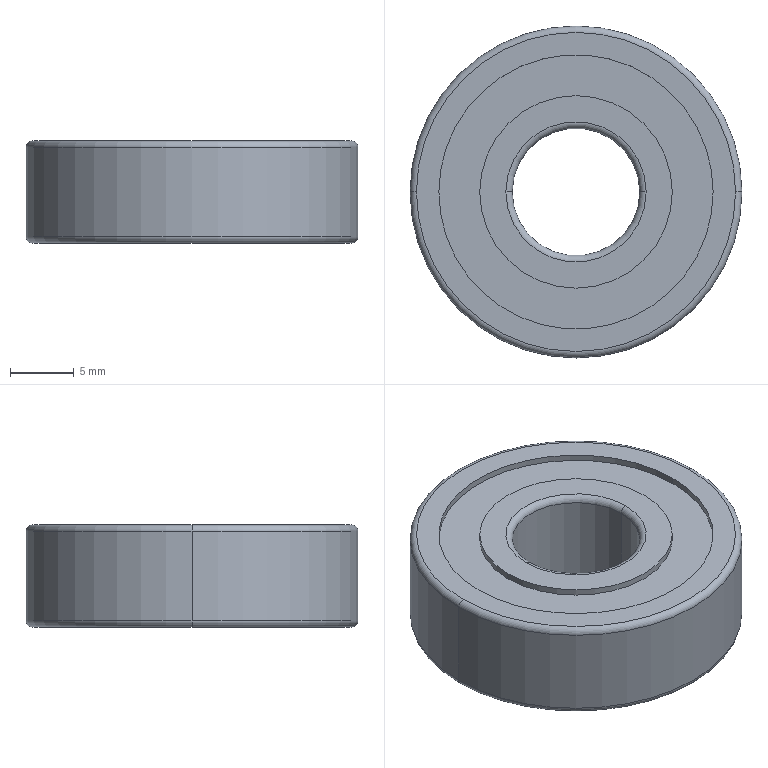Part | NX | features BREP 1 | 1 solid | 26 faces | box 26 x 26 x 8 mm | volume 3423 mm3 | cylinder 12 | torus 8 | plane 6 | commonest cylinder face diameters 15.083 x4 21.486 x4 10 x2 26 x2
STEP:
#1=CARTESIAN_POINT('',(-12.5,0.,4.));
#2=VERTEX_POINT('',#1);
#3=CARTESIAN_POINT('',(12.5,0.,4.));
#4=VERTEX_POINT('',#3);
#5=CARTESIAN_POINT('',(0.,0.,4.));
#6=DIRECTION('',(0.,0.,1.));
#7=DIRECTION('',(-1.,0.,0.));
#8=AXIS2_PLACEMENT_3D('',#5,#6,#7);
#9=CIRCLE('',#8,12.5);
#10=EDGE_CURVE('',#2,#4,#9,.T.);
#11=ORIENTED_EDGE('',*,*,#10,.T.);
#12=CARTESIAN_POINT('',(0.,0.,4.));
#13=DIRECTION('',(0.,0.,1.));
#14=DIRECTION('',(1.,0.,0.));
#15=AXIS2_PLACEMENT_3D('',#12,#13,#14);
#16=CIRCLE('',#15,12.5);
#17=EDGE_CURVE('',#4,#2,#16,.T.);
#18=ORIENTED_EDGE('',*,*,#17,.T.);
#19=EDGE_LOOP('',(#11,#18));
#20=FACE_BOUND('',#19,.T.);
#21=CARTESIAN_POINT('',(10.743,0.,4.));
#22=VERTEX_POINT('',#21);
#23=CARTESIAN_POINT('',(-10.743,0.,4.));
#24=VERTEX_POINT('',#23);
#25=CARTESIAN_POINT('',(0.,0.,4.));
#26=DIRECTION('',(0.,0.,-1.));
#27=DIRECTION('',(1.,0.,0.));
#28=AXIS2_PLACEMENT_3D('',#25,#26,#27);
#29=CIRCLE('',#28,10.743);
#30=EDGE_CURVE('',#22,#24,#29,.T.);
#31=ORIENTED_EDGE('',*,*,#30,.T.);
#32=CARTESIAN_POINT('',(0.,0.,4.));
#33=DIRECTION('',(0.,0.,-1.));
#34=DIRECTION('',(-1.,0.,0.));
#35=AXIS2_PLACEMENT_3D('',#32,#33,#34);
#36=CIRCLE('',#35,10.743);
#37=EDGE_CURVE('',#24,#22,#36,.T.);
#38=ORIENTED_EDGE('',*,*,#37,.T.);
#39=EDGE_LOOP('',(#31,#38));
#40=FACE_BOUND('',#39,.T.);
#41=CARTESIAN_POINT('',(0.,0.,4.));
#42=DIRECTION('',(0.,0.,1.));
#43=DIRECTION('',(-1.,0.,0.));
#44=AXIS2_PLACEMENT_3D('',#41,#42,#43);
#45=PLANE('',#44);
#46=ADVANCED_FACE('',(#20,#40),#45,.T.);
#47=CARTESIAN_POINT('',(-13.,0.,3.5));
#48=VERTEX_POINT('',#47);
#49=CARTESIAN_POINT('',(-12.5,0.,3.5));
#50=DIRECTION('',(0.,-1.,0.));
#51=DIRECTION('',(0.,0.,1.));
#52=AXIS2_PLACEMENT_3D('',#49,#50,#51);
#53=CIRCLE('',#52,0.5);
#54=EDGE_CURVE('',#48,#2,#53,.F.);
#55=ORIENTED_EDGE('',*,*,#54,.T.);
#56=ORIENTED_EDGE('',*,*,#17,.F.);
#57=CARTESIAN_POINT('',(13.,0.,3.5));
#58=VERTEX_POINT('',#57);
#59=CARTESIAN_POINT('',(12.5,0.,3.5));
#60=DIRECTION('',(0.,1.,0.));
#61=DIRECTION('',(0.,0.,1.));
#62=AXIS2_PLACEMENT_3D('',#59,#60,#61);
#63=CIRCLE('',#62,0.5);
#64=EDGE_CURVE('',#58,#4,#63,.F.);
#65=ORIENTED_EDGE('',*,*,#64,.F.);
#66=CARTESIAN_POINT('',(0.,0.,3.5));
#67=DIRECTION('',(0.,0.,1.));
#68=DIRECTION('',(1.,0.,0.));
#69=AXIS2_PLACEMENT_3D('',#66,#67,#68);
#70=CIRCLE('',#69,13.);
#71=EDGE_CURVE('',#58,#48,#70,.T.);
#72=ORIENTED_EDGE('',*,*,#71,.T.);
#73=EDGE_LOOP('',(#55,#56,#65,#72));
#74=FACE_BOUND('',#73,.T.);
#75=CARTESIAN_POINT('',(0.,0.,3.5));
#76=DIRECTION('',(0.,0.,1.));
#77=DIRECTION('',(-1.,0.,0.));
#78=AXIS2_PLACEMENT_3D('',#75,#76,#77);
#79=TOROIDAL_SURFACE('',#78,12.5,0.5);
#80=ADVANCED_FACE('',(#74),#79,.T.);
#81=CARTESIAN_POINT('',(13.,0.,-3.5));
#82=VERTEX_POINT('',#81);
#83=CARTESIAN_POINT('',(13.,0.,-3.5));
#84=DIRECTION('',(0.,0.,1.));
#85=VECTOR('',#84,1000.);
#86=LINE('',#83,#85);
#87=EDGE_CURVE('',#82,#58,#86,.T.);
#88=ORIENTED_EDGE('',*,*,#87,.F.);
#89=CARTESIAN_POINT('',(-13.,0.,-3.5));
#90=VERTEX_POINT('',#89);
#91=CARTESIAN_POINT('',(0.,0.,-3.5));
#92=DIRECTION('',(0.,0.,-1.));
#93=DIRECTION('',(-1.,0.,0.));
#94=AXIS2_PLACEMENT_3D('',#91,#92,#93);
#95=CIRCLE('',#94,13.);
#96=EDGE_CURVE('',#90,#82,#95,.T.);
#97=ORIENTED_EDGE('',*,*,#96,.F.);
#98=CARTESIAN_POINT('',(-13.,0.,-3.5));
#99=DIRECTION('',(0.,0.,1.));
#100=VECTOR('',#99,1000.);
#101=LINE('',#98,#100);
#102=EDGE_CURVE('',#90,#48,#101,.T.);
#103=ORIENTED_EDGE('',*,*,#102,.T.);
#104=ORIENTED_EDGE('',*,*,#71,.F.);
#105=EDGE_LOOP('',(#88,#97,#103,#104));
#106=FACE_BOUND('',#105,.T.);
#107=CARTESIAN_POINT('',(0.,0.,4.));
#108=DIRECTION('',(0.,0.,-1.));
#109=DIRECTION('',(1.,0.,0.));
#110=AXIS2_PLACEMENT_3D('',#107,#108,#109);
#111=CYLINDRICAL_SURFACE('',#110,13.);
#112=ADVANCED_FACE('',(#106),#111,.T.);
#113=CARTESIAN_POINT('',(0.,0.,3.5));
#114=DIRECTION('',(0.,0.,1.));
#115=DIRECTION('',(-1.,0.,0.));
#116=AXIS2_PLACEMENT_3D('',#113,#114,#115);
#117=CIRCLE('',#116,13.);
#118=EDGE_CURVE('',#48,#58,#117,.T.);
#119=ORIENTED_EDGE('',*,*,#118,.F.);
#120=ORIENTED_EDGE('',*,*,#102,.F.);
#121=CARTESIAN_POINT('',(0.,0.,-3.5));
#122=DIRECTION('',(0.,0.,-1.));
#123=DIRECTION('',(1.,0.,0.));
#124=AXIS2_PLACEMENT_3D('',#121,#122,#123);
#125=CIRCLE('',#124,13.);
#126=EDGE_CURVE('',#82,#90,#125,.T.);
#127=ORIENTED_EDGE('',*,*,#126,.F.);
#128=ORIENTED_EDGE('',*,*,#87,.T.);
#129=EDGE_LOOP('',(#119,#120,#127,#128));
#130=FACE_BOUND('',#129,.T.);
#131=CARTESIAN_POINT('',(0.,0.,4.));
#132=DIRECTION('',(0.,0.,-1.));
#133=DIRECTION('',(1.,0.,0.));
#134=AXIS2_PLACEMENT_3D('',#131,#132,#133);
#135=CYLINDRICAL_SURFACE('',#134,13.);
#136=ADVANCED_FACE('',(#130),#135,.T.);
#137=CARTESIAN_POINT('',(12.5,0.,-4.));
#138=VERTEX_POINT('',#137);
#139=CARTESIAN_POINT('',(-12.5,0.,-4.));
#140=VERTEX_POINT('',#139);
#141=CARTESIAN_POINT('',(0.,0.,-4.));
#142=DIRECTION('',(0.,0.,-1.));
#143=DIRECTION('',(1.,0.,0.));
#144=AXIS2_PLACEMENT_3D('',#141,#142,#143);
#145=CIRCLE('',#144,12.5);
#146=EDGE_CURVE('',#138,#140,#145,.T.);
#147=ORIENTED_EDGE('',*,*,#146,.F.);
#148=CARTESIAN_POINT('',(12.5,0.,-3.5));
#149=DIRECTION('',(0.,1.,0.));
#150=DIRECTION('',(1.,0.,0.));
#151=AXIS2_PLACEMENT_3D('',#148,#149,#150);
#152=CIRCLE('',#151,0.5);
#153=EDGE_CURVE('',#82,#138,#152,.T.);
#154=ORIENTED_EDGE('',*,*,#153,.F.);
#155=ORIENTED_EDGE('',*,*,#126,.T.);
#156=CARTESIAN_POINT('',(-12.5,0.,-3.5));
#157=DIRECTION('',(0.,-1.,0.));
#158=DIRECTION('',(-1.,0.,0.));
#159=AXIS2_PLACEMENT_3D('',#156,#157,#158);
#160=CIRCLE('',#159,0.5);
#161=EDGE_CURVE('',#90,#140,#160,.T.);
#162=ORIENTED_EDGE('',*,*,#161,.T.);
#163=EDGE_LOOP('',(#147,#154,#155,#162));
#164=FACE_BOUND('',#163,.T.);
#165=CARTESIAN_POINT('',(0.,0.,-3.5));
#166=DIRECTION('',(0.,0.,1.));
#167=DIRECTION('',(-1.,0.,0.));
#168=AXIS2_PLACEMENT_3D('',#165,#166,#167);
#169=TOROIDAL_SURFACE('',#168,12.5,0.5);
#170=ADVANCED_FACE('',(#164),#169,.T.);
#171=ORIENTED_EDGE('',*,*,#161,.F.);
#172=ORIENTED_EDGE('',*,*,#96,.T.);
#173=ORIENTED_EDGE('',*,*,#153,.T.);
#174=CARTESIAN_POINT('',(0.,0.,-4.));
#175=DIRECTION('',(0.,0.,-1.));
#176=DIRECTION('',(-1.,0.,0.));
#177=AXIS2_PLACEMENT_3D('',#174,#175,#176);
#178=CIRCLE('',#177,12.5);
#179=EDGE_CURVE('',#140,#138,#178,.T.);
#180=ORIENTED_EDGE('',*,*,#179,.F.);
#181=EDGE_LOOP('',(#171,#172,#173,#180));
#182=FACE_BOUND('',#181,.T.);
#183=CARTESIAN_POINT('',(0.,0.,-3.5));
#184=DIRECTION('',(0.,0.,1.));
#185=DIRECTION('',(-1.,0.,0.));
#186=AXIS2_PLACEMENT_3D('',#183,#184,#185);
#187=TOROIDAL_SURFACE('',#186,12.5,0.5);
#188=ADVANCED_FACE('',(#182),#187,.T.);
#189=ORIENTED_EDGE('',*,*,#179,.T.);
#190=ORIENTED_EDGE('',*,*,#146,.T.);
#191=EDGE_LOOP('',(#189,#190));
#192=FACE_BOUND('',#191,.T.);
#193=CARTESIAN_POINT('',(10.743,0.,-4.));
#194=VERTEX_POINT('',#193);
#195=CARTESIAN_POINT('',(-10.743,0.,-4.));
#196=VERTEX_POINT('',#195);
#197=CARTESIAN_POINT('',(0.,0.,-4.));
#198=DIRECTION('',(0.,0.,1.));
#199=DIRECTION('',(1.,0.,0.));
#200=AXIS2_PLACEMENT_3D('',#197,#198,#199);
#201=CIRCLE('',#200,10.743);
#202=EDGE_CURVE('',#194,#196,#201,.T.);
#203=ORIENTED_EDGE('',*,*,#202,.T.);
#204=CARTESIAN_POINT('',(0.,0.,-4.));
#205=DIRECTION('',(0.,0.,1.));
#206=DIRECTION('',(-1.,0.,0.));
#207=AXIS2_PLACEMENT_3D('',#204,#205,#206);
#208=CIRCLE('',#207,10.743);
#209=EDGE_CURVE('',#196,#194,#208,.T.);
#210=ORIENTED_EDGE('',*,*,#209,.T.);
#211=EDGE_LOOP('',(#203,#210));
#212=FACE_BOUND('',#211,.T.);
#213=CARTESIAN_POINT('',(0.,0.,-4.));
#214=DIRECTION('',(0.,0.,1.));
#215=DIRECTION('',(-1.,0.,0.));
#216=AXIS2_PLACEMENT_3D('',#213,#214,#215);
#217=PLANE('',#216);
#218=ADVANCED_FACE('',(#192,#212),#217,.F.);
#219=CARTESIAN_POINT('',(10.743,0.,-3.5));
#220=VERTEX_POINT('',#219);
#221=CARTESIAN_POINT('',(10.743,0.,-4.));
#222=DIRECTION('',(0.,0.,1.));
#223=VECTOR('',#222,1000.);
#224=LINE('',#221,#223);
#225=EDGE_CURVE('',#194,#220,#224,.T.);
#226=ORIENTED_EDGE('',*,*,#225,.F.);
#227=ORIENTED_EDGE('',*,*,#209,.F.);
#228=CARTESIAN_POINT('',(-10.743,0.,-3.5));
#229=VERTEX_POINT('',#228);
#230=CARTESIAN_POINT('',(-10.743,0.,-4.));
#231=DIRECTION('',(0.,0.,1.));
#232=VECTOR('',#231,1000.);
#233=LINE('',#230,#232);
#234=EDGE_CURVE('',#196,#229,#233,.T.);
#235=ORIENTED_EDGE('',*,*,#234,.T.);
#236=CARTESIAN_POINT('',(0.,0.,-3.5));
#237=DIRECTION('',(0.,0.,-1.));
#238=DIRECTION('',(1.,0.,0.));
#239=AXIS2_PLACEMENT_3D('',#236,#237,#238);
#240=CIRCLE('',#239,10.743);
#241=EDGE_CURVE('',#220,#229,#240,.T.);
#242=ORIENTED_EDGE('',*,*,#241,.F.);
#243=EDGE_LOOP('',(#226,#227,#235,#242));
#244=FACE_BOUND('',#243,.T.);
#245=CARTESIAN_POINT('',(0.,0.,-3.5));
#246=DIRECTION('',(0.,0.,-1.));
#247=DIRECTION('',(1.,0.,0.));
#248=AXIS2_PLACEMENT_3D('',#245,#246,#247);
#249=CYLINDRICAL_SURFACE('',#248,10.743);
#250=ADVANCED_FACE('',(#244),#249,.F.);
#251=CARTESIAN_POINT('',(0.,0.,-3.5));
#252=DIRECTION('',(0.,0.,-1.));
#253=DIRECTION('',(-1.,0.,0.));
#254=AXIS2_PLACEMENT_3D('',#251,#252,#253);
#255=CIRCLE('',#254,10.743);
#256=EDGE_CURVE('',#229,#220,#255,.T.);
#257=ORIENTED_EDGE('',*,*,#256,.T.);
#258=ORIENTED_EDGE('',*,*,#241,.T.);
#259=EDGE_LOOP('',(#257,#258));
#260=FACE_BOUND('',#259,.T.);
#261=CARTESIAN_POINT('',(7.542,0.,-3.5));
#262=VERTEX_POINT('',#261);
#263=CARTESIAN_POINT('',(-7.542,0.,-3.5));
#264=VERTEX_POINT('',#263);
#265=CARTESIAN_POINT('',(0.,0.,-3.5));
#266=DIRECTION('',(0.,0.,1.));
#267=DIRECTION('',(1.,0.,0.));
#268=AXIS2_PLACEMENT_3D('',#265,#266,#267);
#269=CIRCLE('',#268,7.542);
#270=EDGE_CURVE('',#262,#264,#269,.T.);
#271=ORIENTED_EDGE('',*,*,#270,.T.);
#272=CARTESIAN_POINT('',(0.,0.,-3.5));
#273=DIRECTION('',(0.,0.,1.));
#274=DIRECTION('',(-1.,0.,0.));
#275=AXIS2_PLACEMENT_3D('',#272,#273,#274);
#276=CIRCLE('',#275,7.542);
#277=EDGE_CURVE('',#264,#262,#276,.T.);
#278=ORIENTED_EDGE('',*,*,#277,.T.);
#279=EDGE_LOOP('',(#271,#278));
#280=FACE_BOUND('',#279,.T.);
#281=CARTESIAN_POINT('',(0.,0.,-3.5));
#282=DIRECTION('',(0.,0.,-1.));
#283=DIRECTION('',(-1.,0.,0.));
#284=AXIS2_PLACEMENT_3D('',#281,#282,#283);
#285=PLANE('',#284);
#286=ADVANCED_FACE('',(#260,#280),#285,.T.);
#287=ORIENTED_EDGE('',*,*,#256,.F.);
#288=ORIENTED_EDGE('',*,*,#234,.F.);
#289=ORIENTED_EDGE('',*,*,#202,.F.);
#290=ORIENTED_EDGE('',*,*,#225,.T.);
#291=EDGE_LOOP('',(#287,#288,#289,#290));
#292=FACE_BOUND('',#291,.T.);
#293=CARTESIAN_POINT('',(0.,0.,-3.5));
#294=DIRECTION('',(0.,0.,-1.));
#295=DIRECTION('',(1.,0.,0.));
#296=AXIS2_PLACEMENT_3D('',#293,#294,#295);
#297=CYLINDRICAL_SURFACE('',#296,10.743);
#298=ADVANCED_FACE('',(#292),#297,.F.);
#299=ORIENTED_EDGE('',*,*,#277,.F.);
#300=CARTESIAN_POINT('',(-7.542,0.,-4.));
#301=VERTEX_POINT('',#300);
#302=CARTESIAN_POINT('',(-7.542,0.,-4.));
#303=DIRECTION('',(0.,0.,1.));
#304=VECTOR('',#303,1000.);
#305=LINE('',#302,#304);
#306=EDGE_CURVE('',#264,#301,#305,.F.);
#307=ORIENTED_EDGE('',*,*,#306,.T.);
#308=CARTESIAN_POINT('',(7.542,0.,-4.));
#309=VERTEX_POINT('',#308);
#310=CARTESIAN_POINT('',(0.,0.,-4.));
#311=DIRECTION('',(0.,0.,-1.));
#312=DIRECTION('',(1.,0.,0.));
#313=AXIS2_PLACEMENT_3D('',#310,#311,#312);
#314=CIRCLE('',#313,7.542);
#315=EDGE_CURVE('',#309,#301,#314,.T.);
#316=ORIENTED_EDGE('',*,*,#315,.F.);
#317=CARTESIAN_POINT('',(7.542,0.,-4.));
#318=DIRECTION('',(0.,0.,1.));
#319=VECTOR('',#318,1000.);
#320=LINE('',#317,#319);
#321=EDGE_CURVE('',#262,#309,#320,.F.);
#322=ORIENTED_EDGE('',*,*,#321,.F.);
#323=EDGE_LOOP('',(#299,#307,#316,#322));
#324=FACE_BOUND('',#323,.T.);
#325=CARTESIAN_POINT('',(0.,0.,-3.5));
#326=DIRECTION('',(0.,0.,-1.));
#327=DIRECTION('',(1.,0.,0.));
#328=AXIS2_PLACEMENT_3D('',#325,#326,#327);
#329=CYLINDRICAL_SURFACE('',#328,7.542);
#330=ADVANCED_FACE('',(#324),#329,.T.);
#331=ORIENTED_EDGE('',*,*,#321,.T.);
#332=CARTESIAN_POINT('',(0.,0.,-4.));
#333=DIRECTION('',(0.,0.,-1.));
#334=DIRECTION('',(-1.,0.,0.));
#335=AXIS2_PLACEMENT_3D('',#332,#333,#334);
#336=CIRCLE('',#335,7.542);
#337=EDGE_CURVE('',#301,#309,#336,.T.);
#338=ORIENTED_EDGE('',*,*,#337,.F.);
#339=ORIENTED_EDGE('',*,*,#306,.F.);
#340=ORIENTED_EDGE('',*,*,#270,.F.);
#341=EDGE_LOOP('',(#331,#338,#339,#340));
#342=FACE_BOUND('',#341,.T.);
#343=CARTESIAN_POINT('',(0.,0.,-3.5));
#344=DIRECTION('',(0.,0.,-1.));
#345=DIRECTION('',(1.,0.,0.));
#346=AXIS2_PLACEMENT_3D('',#343,#344,#345);
#347=CYLINDRICAL_SURFACE('',#346,7.542);
#348=ADVANCED_FACE('',(#342),#347,.T.);
#349=ORIENTED_EDGE('',*,*,#337,.T.);
#350=ORIENTED_EDGE('',*,*,#315,.T.);
#351=EDGE_LOOP('',(#349,#350));
#352=FACE_BOUND('',#351,.T.);
#353=CARTESIAN_POINT('',(-5.5,0.,-4.));
#354=VERTEX_POINT('',#353);
#355=CARTESIAN_POINT('',(5.5,0.,-4.));
#356=VERTEX_POINT('',#355);
#357=CARTESIAN_POINT('',(0.,0.,-4.));
#358=DIRECTION('',(0.,0.,1.));
#359=DIRECTION('',(-1.,0.,0.));
#360=AXIS2_PLACEMENT_3D('',#357,#358,#359);
#361=CIRCLE('',#360,5.5);
#362=EDGE_CURVE('',#354,#356,#361,.T.);
#363=ORIENTED_EDGE('',*,*,#362,.T.);
#364=CARTESIAN_POINT('',(0.,0.,-4.));
#365=DIRECTION('',(0.,0.,1.));
#366=DIRECTION('',(1.,0.,0.));
#367=AXIS2_PLACEMENT_3D('',#364,#365,#366);
#368=CIRCLE('',#367,5.5);
#369=EDGE_CURVE('',#356,#354,#368,.T.);
#370=ORIENTED_EDGE('',*,*,#369,.T.);
#371=EDGE_LOOP('',(#363,#370));
#372=FACE_BOUND('',#371,.T.);
#373=CARTESIAN_POINT('',(0.,0.,-4.));
#374=DIRECTION('',(0.,0.,1.));
#375=DIRECTION('',(-1.,0.,0.));
#376=AXIS2_PLACEMENT_3D('',#373,#374,#375);
#377=PLANE('',#376);
#378=ADVANCED_FACE('',(#352,#372),#377,.F.);
#379=CARTESIAN_POINT('',(-5.,0.,-3.5));
#380=VERTEX_POINT('',#379);
#381=CARTESIAN_POINT('',(-5.5,0.,-3.5));
#382=DIRECTION('',(0.,-1.,0.));
#383=DIRECTION('',(0.,0.,-1.));
#384=AXIS2_PLACEMENT_3D('',#381,#382,#383);
#385=CIRCLE('',#384,0.5);
#386=EDGE_CURVE('',#380,#354,#385,.F.);
#387=ORIENTED_EDGE('',*,*,#386,.T.);
#388=ORIENTED_EDGE('',*,*,#369,.F.);
#389=CARTESIAN_POINT('',(5.,0.,-3.5));
#390=VERTEX_POINT('',#389);
#391=CARTESIAN_POINT('',(5.5,0.,-3.5));
#392=DIRECTION('',(0.,1.,0.));
#393=DIRECTION('',(0.,0.,-1.));
#394=AXIS2_PLACEMENT_3D('',#391,#392,#393);
#395=CIRCLE('',#394,0.5);
#396=EDGE_CURVE('',#390,#356,#395,.F.);
#397=ORIENTED_EDGE('',*,*,#396,.F.);
#398=CARTESIAN_POINT('',(0.,0.,-3.5));
#399=DIRECTION('',(0.,0.,1.));
#400=DIRECTION('',(1.,0.,0.));
#401=AXIS2_PLACEMENT_3D('',#398,#399,#400);
#402=CIRCLE('',#401,5.);
#403=EDGE_CURVE('',#390,#380,#402,.T.);
#404=ORIENTED_EDGE('',*,*,#403,.T.);
#405=EDGE_LOOP('',(#387,#388,#397,#404));
#406=FACE_BOUND('',#405,.T.);
#407=CARTESIAN_POINT('',(0.,0.,-3.5));
#408=DIRECTION('',(0.,0.,1.));
#409=DIRECTION('',(-1.,0.,0.));
#410=AXIS2_PLACEMENT_3D('',#407,#408,#409);
#411=TOROIDAL_SURFACE('',#410,5.5,0.5);
#412=ADVANCED_FACE('',(#406),#411,.T.);
#413=CARTESIAN_POINT('',(-5.,0.,3.5));
#414=VERTEX_POINT('',#413);
#415=CARTESIAN_POINT('',(5.,0.,3.5));
#416=VERTEX_POINT('',#415);
#417=CARTESIAN_POINT('',(0.,0.,3.5));
#418=DIRECTION('',(0.,0.,-1.));
#419=DIRECTION('',(-1.,0.,0.));
#420=AXIS2_PLACEMENT_3D('',#417,#418,#419);
#421=CIRCLE('',#420,5.);
#422=EDGE_CURVE('',#414,#416,#421,.T.);
#423=ORIENTED_EDGE('',*,*,#422,.F.);
#424=CARTESIAN_POINT('',(-5.,0.,-3.5));
#425=DIRECTION('',(0.,0.,1.));
#426=VECTOR('',#425,1000.);
#427=LINE('',#424,#426);
#428=EDGE_CURVE('',#414,#380,#427,.F.);
#429=ORIENTED_EDGE('',*,*,#428,.T.);
#430=ORIENTED_EDGE('',*,*,#403,.F.);
#431=CARTESIAN_POINT('',(5.,0.,-3.5));
#432=DIRECTION('',(0.,0.,1.));
#433=VECTOR('',#432,1000.);
#434=LINE('',#431,#433);
#435=EDGE_CURVE('',#416,#390,#434,.F.);
#436=ORIENTED_EDGE('',*,*,#435,.F.);
#437=EDGE_LOOP('',(#423,#429,#430,#436));
#438=FACE_BOUND('',#437,.T.);
#439=CARTESIAN_POINT('',(0.,0.,4.));
#440=DIRECTION('',(0.,0.,-1.));
#441=DIRECTION('',(1.,0.,0.));
#442=AXIS2_PLACEMENT_3D('',#439,#440,#441);
#443=CYLINDRICAL_SURFACE('',#442,5.);
#444=ADVANCED_FACE('',(#438),#443,.F.);
#445=ORIENTED_EDGE('',*,*,#435,.T.);
#446=CARTESIAN_POINT('',(0.,0.,-3.5));
#447=DIRECTION('',(0.,0.,1.));
#448=DIRECTION('',(-1.,0.,0.));
#449=AXIS2_PLACEMENT_3D('',#446,#447,#448);
#450=CIRCLE('',#449,5.);
#451=EDGE_CURVE('',#380,#390,#450,.T.);
#452=ORIENTED_EDGE('',*,*,#451,.F.);
#453=ORIENTED_EDGE('',*,*,#428,.F.);
#454=CARTESIAN_POINT('',(0.,0.,3.5));
#455=DIRECTION('',(0.,0.,-1.));
#456=DIRECTION('',(1.,0.,0.));
#457=AXIS2_PLACEMENT_3D('',#454,#455,#456);
#458=CIRCLE('',#457,5.);
#459=EDGE_CURVE('',#416,#414,#458,.T.);
#460=ORIENTED_EDGE('',*,*,#459,.F.);
#461=EDGE_LOOP('',(#445,#452,#453,#460));
#462=FACE_BOUND('',#461,.T.);
#463=CARTESIAN_POINT('',(0.,0.,4.));
#464=DIRECTION('',(0.,0.,-1.));
#465=DIRECTION('',(1.,0.,0.));
#466=AXIS2_PLACEMENT_3D('',#463,#464,#465);
#467=CYLINDRICAL_SURFACE('',#466,5.);
#468=ADVANCED_FACE('',(#462),#467,.F.);
#469=CARTESIAN_POINT('',(5.5,0.,4.));
#470=VERTEX_POINT('',#469);
#471=CARTESIAN_POINT('',(-5.5,0.,4.));
#472=VERTEX_POINT('',#471);
#473=CARTESIAN_POINT('',(0.,0.,4.));
#474=DIRECTION('',(0.,0.,-1.));
#475=DIRECTION('',(1.,0.,0.));
#476=AXIS2_PLACEMENT_3D('',#473,#474,#475);
#477=CIRCLE('',#476,5.5);
#478=EDGE_CURVE('',#470,#472,#477,.T.);
#479=ORIENTED_EDGE('',*,*,#478,.F.);
#480=CARTESIAN_POINT('',(5.5,0.,3.5));
#481=DIRECTION('',(0.,1.,0.));
#482=DIRECTION('',(-1.,0.,0.));
#483=AXIS2_PLACEMENT_3D('',#480,#481,#482);
#484=CIRCLE('',#483,0.5);
#485=EDGE_CURVE('',#416,#470,#484,.T.);
#486=ORIENTED_EDGE('',*,*,#485,.F.);
#487=ORIENTED_EDGE('',*,*,#459,.T.);
#488=CARTESIAN_POINT('',(-5.5,0.,3.5));
#489=DIRECTION('',(0.,-1.,0.));
#490=DIRECTION('',(1.,0.,0.));
#491=AXIS2_PLACEMENT_3D('',#488,#489,#490);
#492=CIRCLE('',#491,0.5);
#493=EDGE_CURVE('',#414,#472,#492,.T.);
#494=ORIENTED_EDGE('',*,*,#493,.T.);
#495=EDGE_LOOP('',(#479,#486,#487,#494));
#496=FACE_BOUND('',#495,.T.);
#497=CARTESIAN_POINT('',(0.,0.,3.5));
#498=DIRECTION('',(0.,0.,1.));
#499=DIRECTION('',(-1.,0.,0.));
#500=AXIS2_PLACEMENT_3D('',#497,#498,#499);
#501=TOROIDAL_SURFACE('',#500,5.5,0.5);
#502=ADVANCED_FACE('',(#496),#501,.T.);
#503=ORIENTED_EDGE('',*,*,#493,.F.);
#504=ORIENTED_EDGE('',*,*,#422,.T.);
#505=ORIENTED_EDGE('',*,*,#485,.T.);
#506=CARTESIAN_POINT('',(0.,0.,4.));
#507=DIRECTION('',(0.,0.,-1.));
#508=DIRECTION('',(-1.,0.,0.));
#509=AXIS2_PLACEMENT_3D('',#506,#507,#508);
#510=CIRCLE('',#509,5.5);
#511=EDGE_CURVE('',#472,#470,#510,.T.);
#512=ORIENTED_EDGE('',*,*,#511,.F.);
#513=EDGE_LOOP('',(#503,#504,#505,#512));
#514=FACE_BOUND('',#513,.T.);
#515=CARTESIAN_POINT('',(0.,0.,3.5));
#516=DIRECTION('',(0.,0.,1.));
#517=DIRECTION('',(-1.,0.,0.));
#518=AXIS2_PLACEMENT_3D('',#515,#516,#517);
#519=TOROIDAL_SURFACE('',#518,5.5,0.5);
#520=ADVANCED_FACE('',(#514),#519,.T.);
#521=CARTESIAN_POINT('',(-7.542,0.,4.));
#522=VERTEX_POINT('',#521);
#523=CARTESIAN_POINT('',(7.542,0.,4.));
#524=VERTEX_POINT('',#523);
#525=CARTESIAN_POINT('',(0.,0.,4.));
#526=DIRECTION('',(0.,0.,1.));
#527=DIRECTION('',(-1.,0.,0.));
#528=AXIS2_PLACEMENT_3D('',#525,#526,#527);
#529=CIRCLE('',#528,7.542);
#530=EDGE_CURVE('',#522,#524,#529,.T.);
#531=ORIENTED_EDGE('',*,*,#530,.T.);
#532=CARTESIAN_POINT('',(0.,0.,4.));
#533=DIRECTION('',(0.,0.,1.));
#534=DIRECTION('',(1.,0.,0.));
#535=AXIS2_PLACEMENT_3D('',#532,#533,#534);
#536=CIRCLE('',#535,7.542);
#537=EDGE_CURVE('',#524,#522,#536,.T.);
#538=ORIENTED_EDGE('',*,*,#537,.T.);
#539=EDGE_LOOP('',(#531,#538));
#540=FACE_BOUND('',#539,.T.);
#541=ORIENTED_EDGE('',*,*,#511,.T.);
#542=ORIENTED_EDGE('',*,*,#478,.T.);
#543=EDGE_LOOP('',(#541,#542));
#544=FACE_BOUND('',#543,.T.);
#545=CARTESIAN_POINT('',(0.,0.,4.));
#546=DIRECTION('',(0.,0.,1.));
#547=DIRECTION('',(-1.,0.,0.));
#548=AXIS2_PLACEMENT_3D('',#545,#546,#547);
#549=PLANE('',#548);
#550=ADVANCED_FACE('',(#540,#544),#549,.T.);
#551=CARTESIAN_POINT('',(-7.542,0.,3.5));
#552=VERTEX_POINT('',#551);
#553=CARTESIAN_POINT('',(-7.542,0.,4.));
#554=DIRECTION('',(0.,0.,-1.));
#555=VECTOR('',#554,1000.);
#556=LINE('',#553,#555);
#557=EDGE_CURVE('',#552,#522,#556,.F.);
#558=ORIENTED_EDGE('',*,*,#557,.T.);
#559=ORIENTED_EDGE('',*,*,#537,.F.);
#560=CARTESIAN_POINT('',(7.542,0.,3.5));
#561=VERTEX_POINT('',#560);
#562=CARTESIAN_POINT('',(7.542,0.,4.));
#563=DIRECTION('',(0.,0.,-1.));
#564=VECTOR('',#563,1000.);
#565=LINE('',#562,#564);
#566=EDGE_CURVE('',#561,#524,#565,.F.);
#567=ORIENTED_EDGE('',*,*,#566,.F.);
#568=CARTESIAN_POINT('',(0.,0.,3.5));
#569=DIRECTION('',(0.,0.,-1.));
#570=DIRECTION('',(-1.,0.,0.));
#571=AXIS2_PLACEMENT_3D('',#568,#569,#570);
#572=CIRCLE('',#571,7.542);
#573=EDGE_CURVE('',#552,#561,#572,.T.);
#574=ORIENTED_EDGE('',*,*,#573,.F.);
#575=EDGE_LOOP('',(#558,#559,#567,#574));
#576=FACE_BOUND('',#575,.T.);
#577=CARTESIAN_POINT('',(0.,0.,3.5));
#578=DIRECTION('',(0.,0.,1.));
#579=DIRECTION('',(-1.,0.,0.));
#580=AXIS2_PLACEMENT_3D('',#577,#578,#579);
#581=CYLINDRICAL_SURFACE('',#580,7.542);
#582=ADVANCED_FACE('',(#576),#581,.T.);
#583=CARTESIAN_POINT('',(-10.743,0.,3.5));
#584=VERTEX_POINT('',#583);
#585=CARTESIAN_POINT('',(10.743,0.,3.5));
#586=VERTEX_POINT('',#585);
#587=CARTESIAN_POINT('',(0.,0.,3.5));
#588=DIRECTION('',(0.,0.,1.));
#589=DIRECTION('',(-1.,0.,0.));
#590=AXIS2_PLACEMENT_3D('',#587,#588,#589);
#591=CIRCLE('',#590,10.743);
#592=EDGE_CURVE('',#584,#586,#591,.T.);
#593=ORIENTED_EDGE('',*,*,#592,.T.);
#594=CARTESIAN_POINT('',(0.,0.,3.5));
#595=DIRECTION('',(0.,0.,1.));
#596=DIRECTION('',(1.,0.,0.));
#597=AXIS2_PLACEMENT_3D('',#594,#595,#596);
#598=CIRCLE('',#597,10.743);
#599=EDGE_CURVE('',#586,#584,#598,.T.);
#600=ORIENTED_EDGE('',*,*,#599,.T.);
#601=EDGE_LOOP('',(#593,#600));
#602=FACE_BOUND('',#601,.T.);
#603=CARTESIAN_POINT('',(0.,0.,3.5));
#604=DIRECTION('',(0.,0.,-1.));
#605=DIRECTION('',(1.,0.,0.));
#606=AXIS2_PLACEMENT_3D('',#603,#604,#605);
#607=CIRCLE('',#606,7.542);
#608=EDGE_CURVE('',#561,#552,#607,.T.);
#609=ORIENTED_EDGE('',*,*,#608,.T.);
#610=ORIENTED_EDGE('',*,*,#573,.T.);
#611=EDGE_LOOP('',(#609,#610));
#612=FACE_BOUND('',#611,.T.);
#613=CARTESIAN_POINT('',(0.,0.,3.5));
#614=DIRECTION('',(0.,0.,1.));
#615=DIRECTION('',(-1.,0.,0.));
#616=AXIS2_PLACEMENT_3D('',#613,#614,#615);
#617=PLANE('',#616);
#618=ADVANCED_FACE('',(#602,#612),#617,.T.);
#619=ORIENTED_EDGE('',*,*,#599,.F.);
#620=CARTESIAN_POINT('',(10.743,0.,4.));
#621=DIRECTION('',(0.,0.,-1.));
#622=VECTOR('',#621,1000.);
#623=LINE('',#620,#622);
#624=EDGE_CURVE('',#22,#586,#623,.T.);
#625=ORIENTED_EDGE('',*,*,#624,.F.);
#626=ORIENTED_EDGE('',*,*,#37,.F.);
#627=CARTESIAN_POINT('',(-10.743,0.,4.));
#628=DIRECTION('',(0.,0.,-1.));
#629=VECTOR('',#628,1000.);
#630=LINE('',#627,#629);
#631=EDGE_CURVE('',#24,#584,#630,.T.);
#632=ORIENTED_EDGE('',*,*,#631,.T.);
#633=EDGE_LOOP('',(#619,#625,#626,#632));
#634=FACE_BOUND('',#633,.T.);
#635=CARTESIAN_POINT('',(0.,0.,3.5));
#636=DIRECTION('',(0.,0.,1.));
#637=DIRECTION('',(-1.,0.,0.));
#638=AXIS2_PLACEMENT_3D('',#635,#636,#637);
#639=CYLINDRICAL_SURFACE('',#638,10.743);
#640=ADVANCED_FACE('',(#634),#639,.F.);
#641=ORIENTED_EDGE('',*,*,#631,.F.);
#642=ORIENTED_EDGE('',*,*,#30,.F.);
#643=ORIENTED_EDGE('',*,*,#624,.T.);
#644=ORIENTED_EDGE('',*,*,#592,.F.);
#645=EDGE_LOOP('',(#641,#642,#643,#644));
#646=FACE_BOUND('',#645,.T.);
#647=CARTESIAN_POINT('',(0.,0.,3.5));
#648=DIRECTION('',(0.,0.,1.));
#649=DIRECTION('',(-1.,0.,0.));
#650=AXIS2_PLACEMENT_3D('',#647,#648,#649);
#651=CYLINDRICAL_SURFACE('',#650,10.743);
#652=ADVANCED_FACE('',(#646),#651,.F.);
#653=ORIENTED_EDGE('',*,*,#608,.F.);
#654=ORIENTED_EDGE('',*,*,#566,.T.);
#655=ORIENTED_EDGE('',*,*,#530,.F.);
#656=ORIENTED_EDGE('',*,*,#557,.F.);
#657=EDGE_LOOP('',(#653,#654,#655,#656));
#658=FACE_BOUND('',#657,.T.);
#659=CARTESIAN_POINT('',(0.,0.,3.5));
#660=DIRECTION('',(0.,0.,1.));
#661=DIRECTION('',(-1.,0.,0.));
#662=AXIS2_PLACEMENT_3D('',#659,#660,#661);
#663=CYLINDRICAL_SURFACE('',#662,7.542);
#664=ADVANCED_FACE('',(#658),#663,.T.);
#665=ORIENTED_EDGE('',*,*,#451,.T.);
#666=ORIENTED_EDGE('',*,*,#396,.T.);
#667=ORIENTED_EDGE('',*,*,#362,.F.);
#668=ORIENTED_EDGE('',*,*,#386,.F.);
#669=EDGE_LOOP('',(#665,#666,#667,#668));
#670=FACE_BOUND('',#669,.T.);
#671=CARTESIAN_POINT('',(0.,0.,-3.5));
#672=DIRECTION('',(0.,0.,1.));
#673=DIRECTION('',(-1.,0.,0.));
#674=AXIS2_PLACEMENT_3D('',#671,#672,#673);
#675=TOROIDAL_SURFACE('',#674,5.5,0.5);
#676=ADVANCED_FACE('',(#670),#675,.T.);
#677=ORIENTED_EDGE('',*,*,#118,.T.);
#678=ORIENTED_EDGE('',*,*,#64,.T.);
#679=ORIENTED_EDGE('',*,*,#10,.F.);
#680=ORIENTED_EDGE('',*,*,#54,.F.);
#681=EDGE_LOOP('',(#677,#678,#679,#680));
#682=FACE_BOUND('',#681,.T.);
#683=CARTESIAN_POINT('',(0.,0.,3.5));
#684=DIRECTION('',(0.,0.,1.));
#685=DIRECTION('',(-1.,0.,0.));
#686=AXIS2_PLACEMENT_3D('',#683,#684,#685);
#687=TOROIDAL_SURFACE('',#686,12.5,0.5);
#688=ADVANCED_FACE('',(#682),#687,.T.);
#689=CLOSED_SHELL('',(#46,#80,#112,#136,#170,#188,#218,#250,#286,#298,#330,#348,#378,#412,#444,#468,#502,#520,#550,#582,#618,#640,#652,#664,#676,#688));
#690=MANIFOLD_SOLID_BREP('',#689);
#691=(LENGTH_UNIT()NAMED_UNIT(*)SI_UNIT(.MILLI.,.METRE.));
#692=UNCERTAINTY_MEASURE_WITH_UNIT(LENGTH_MEASURE(0.00001),#691,'','');
#693=(NAMED_UNIT(*)PLANE_ANGLE_UNIT()SI_UNIT($,.RADIAN.));
#694=(NAMED_UNIT(*)SI_UNIT($,.STERADIAN.)SOLID_ANGLE_UNIT());
#695=(GEOMETRIC_REPRESENTATION_CONTEXT(3)GLOBAL_UNCERTAINTY_ASSIGNED_CONTEXT((#692))GLOBAL_UNIT_ASSIGNED_CONTEXT((#691,#693,#694))REPRESENTATION_CONTEXT('',''));
#696=ADVANCED_BREP_SHAPE_REPRESENTATION('',(#690),#695);